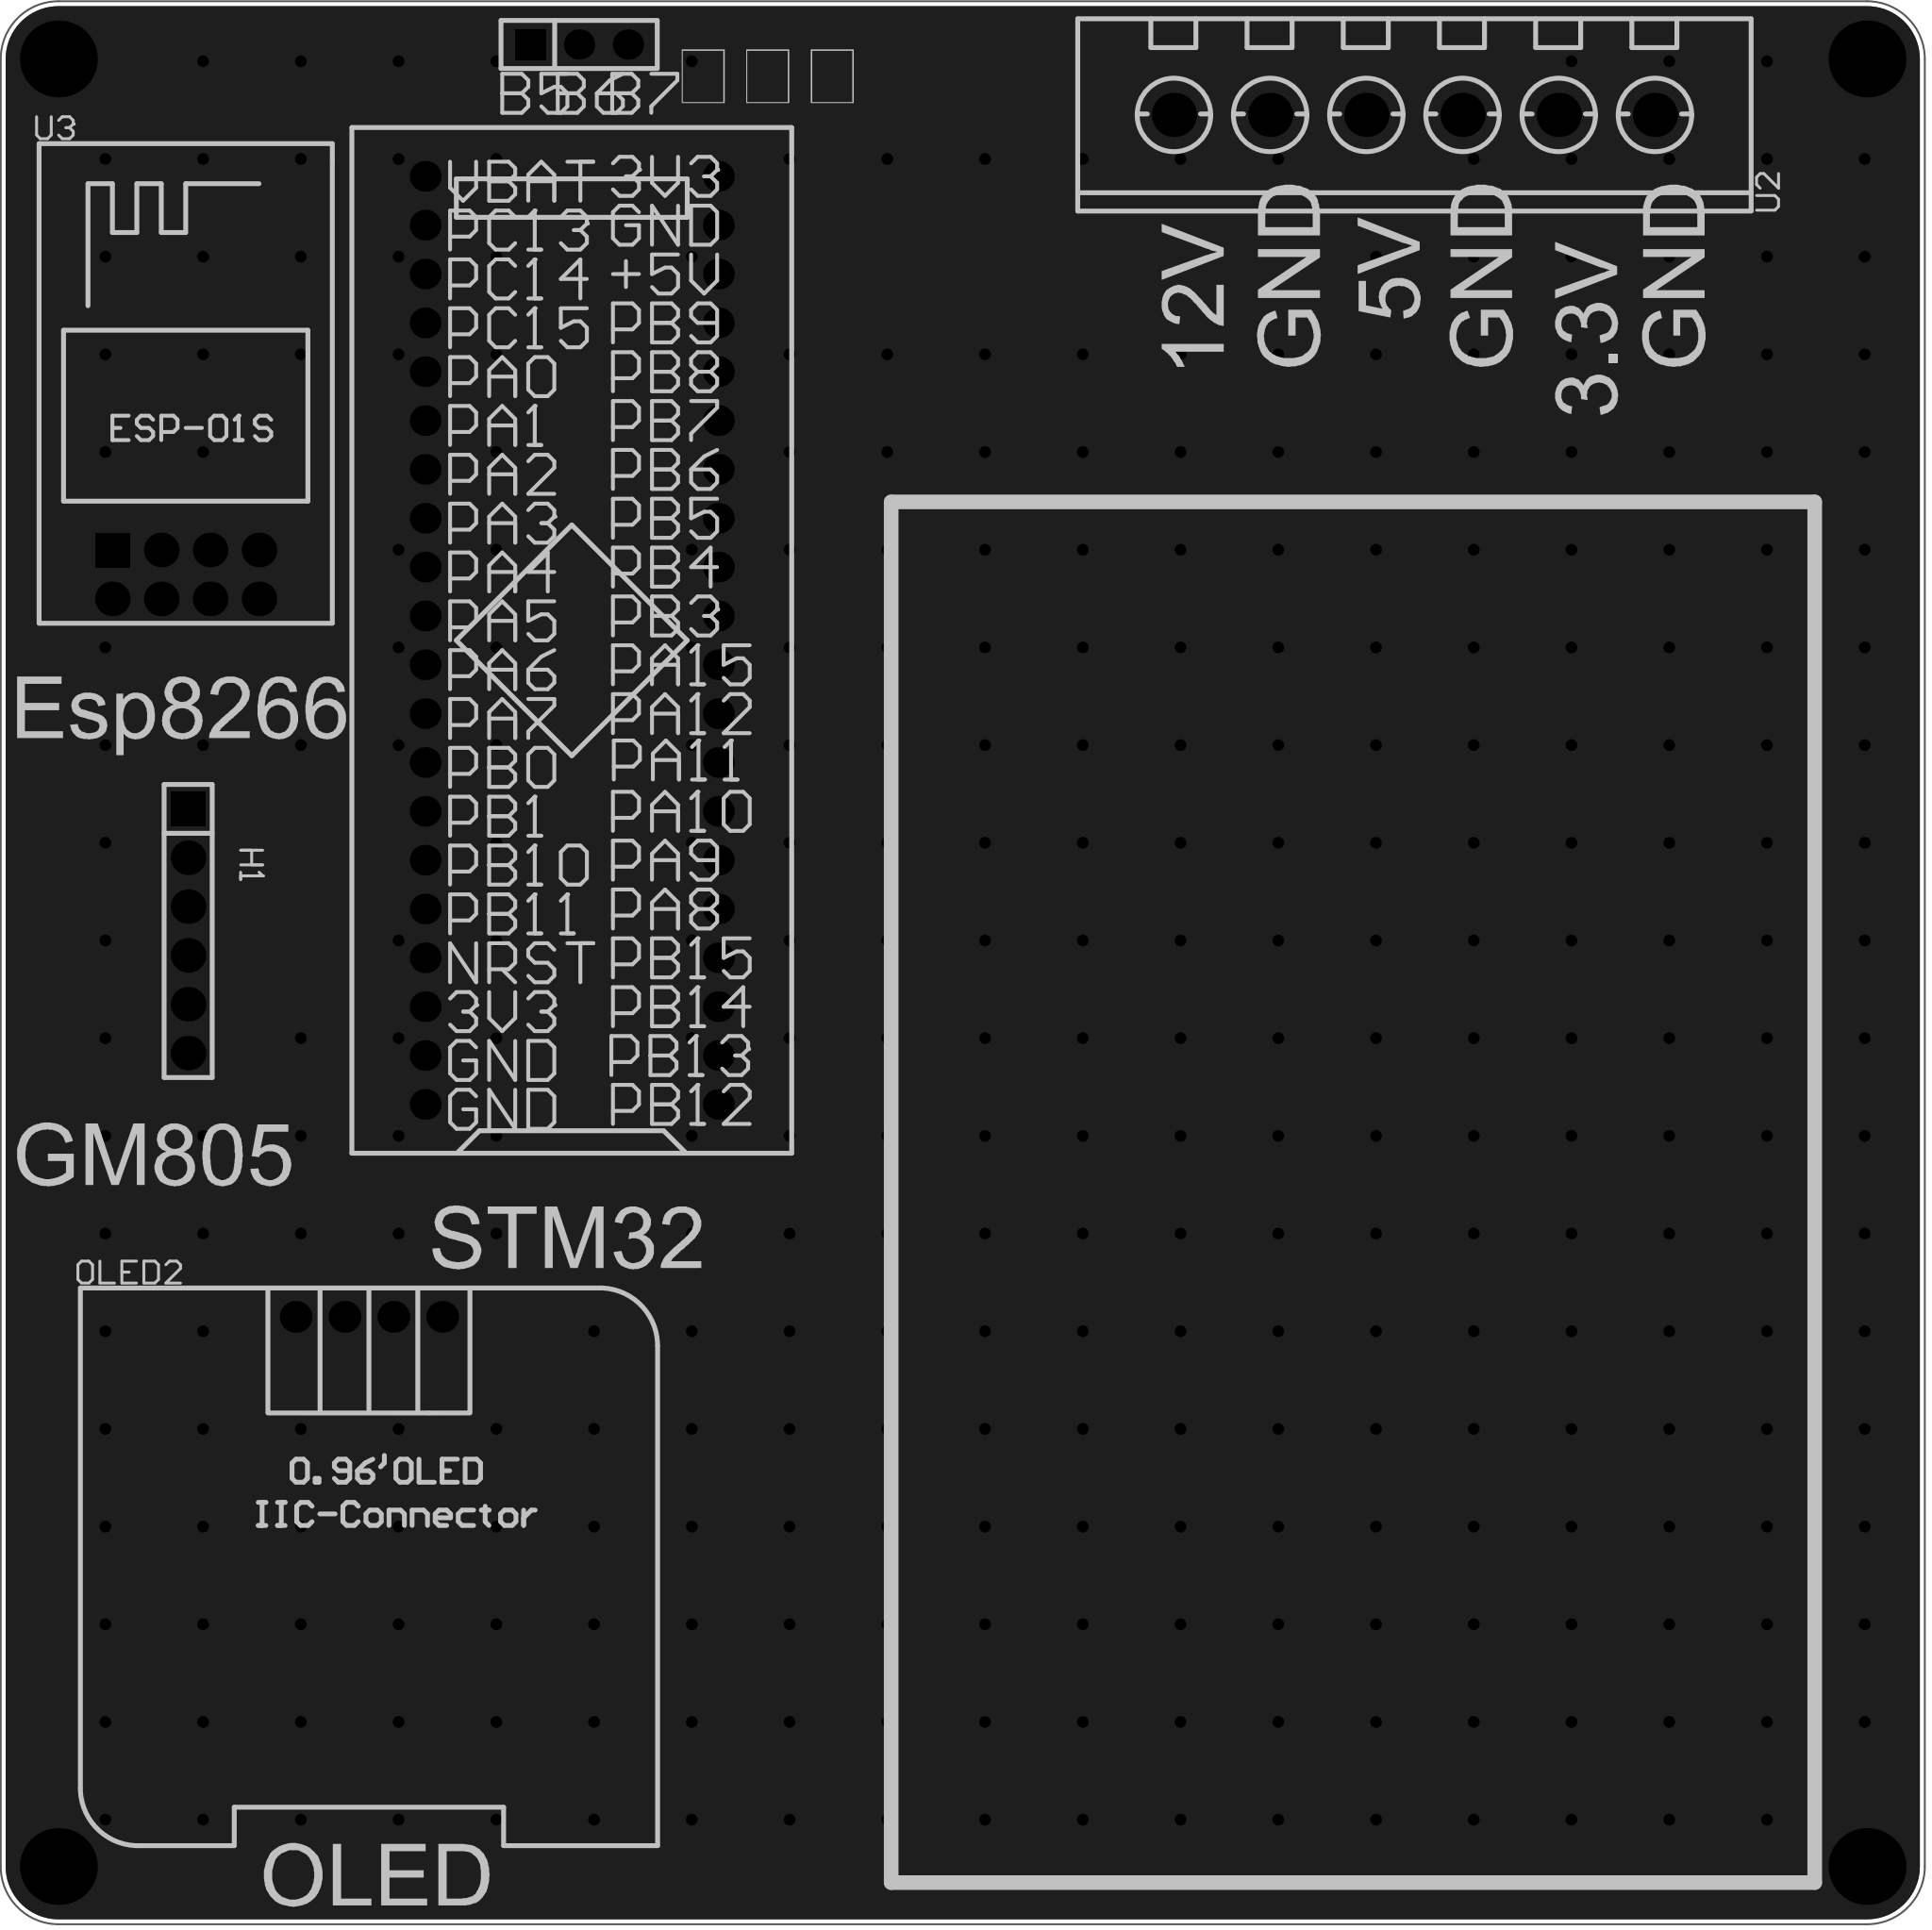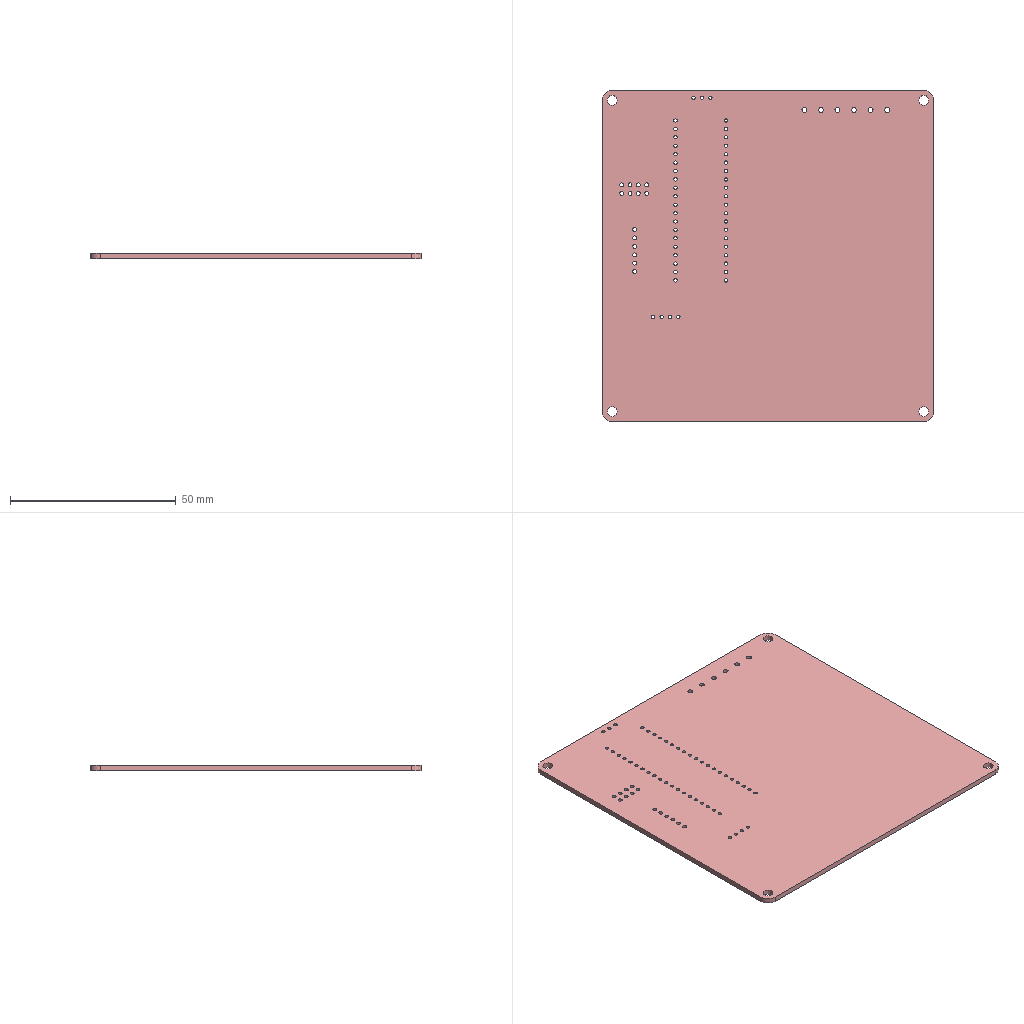Circuit board layout | Altium Designer | box 100 x 100 x 1.6 mm
Layer stack:
# Altium Designer layer stack of  (unit mm; dielectric type: 0 none, 1 core, 2 prepreg, 3 surface material)
index,name,kind,layer,copper_thickness_mm,dielectric_type,dielectric_thickness_mm,dielectric_material,dielectric_constant
0,Top Paste Mask Layer,other,,,,,,
1,Top Silkscreen Layer,other,,,,,,
2,Top Solder Mask Layer,dielectric,,,3,0.01,,3.3
3,Top Layer,copper,Top Layer,0.035,,,,
4,Dielectric1,dielectric,,,3,1.51,FR4,4.5
5,Bottom Layer,copper,Bottom Layer,0.035,,,,
6,Bottom Solder Mask Layer,dielectric,,,3,0.01,,3.3
7,Bottom Silkscreen Layer,other,,,,,,
8,Bottom Paste Mask Layer,other,,,,,,
# drill layer pairs: low layer,high layer
drill_pair,Top Layer,Bottom Layer
Part placement:
Designator,Comment,Layer,Footprint,Center-X(mm),Center-Y(mm),Rotation
U1,STM32F103C8T6-Card,TopLayer,CONN-TH_L53.3-W22.9_STM32F103C8T6-CARD,121.031,149.479,90
OLED2,,TopLayer,0.96OLED_4P,110.49,114.3,0
H9,,TopLayer,HDR-TH_3P-P2.54-V-F,121.412,180.467,0
U3,ESP-01S,TopLayer,WIFIM-TH_ESP-01S,100.965,152.908,0
U2,LG128V 5.08 6P180度螺丝用十字带一字型,TopLayer,CONN-TH_6P-P5.00_LG128V,164.826,176.804,180
H1,,TopLayer,HDR-TH_6P-P2.54-V-M-1,101.092,134.366,270
Pad and via stacks:
# Altium Designer via and pad stacks of  (unit mm). Each distinct definition once, with the count of objects using it.
# via: kind,start_layer,end_layer,hole_mm,diameter_mm,mode(0 simple;1 top-mid-bottom;2 full stack),diameter_per_layer,count,example_net
# pad: kind,layer,hole_mm,hole_type(0 round;1 square;2 slot),plating,top_size,top_shape(1 round;2 rect;3 octagon;9 rounded rect),mid_size,bottom_size,mode,footprint,size_per_layer,count,example
pad,Multi-Layer,3,0,plated,4x4,1,4x4,4x4,0,,,4,1
pad,Multi-Layer,1,0,plated,1.6x1.6,1,1.6x1.6,1.6x1.6,0,CONN-TH_L53.3-W22.9_STM32F103C8T6-CARD,,40,U1.1
pad,Multi-Layer,1,0,plated,1.65x1.65,1,1.65x1.65,1.65x1.65,0,0.96OLED_4P,,4,OLED2.4
pad,Multi-Layer,1.02,0,plated,1.575x1.575,1,1.575x1.575,1.575x1.575,0,HDR-TH_3P-P2.54-V-F,,2,H9.3
pad,Multi-Layer,1.02,0,plated,1.575x1.575,2,1.575x1.575,1.575x1.575,0,HDR-TH_3P-P2.54-V-F,,1,H9.1
pad,Multi-Layer,1.2,0,plated,1.8x1.8,2,1.8x1.8,1.8x1.8,0,WIFIM-TH_ESP-01S,,1,U3.1
pad,Multi-Layer,1.2,0,plated,1.8x1.8,1,1.8x1.8,1.8x1.8,0,WIFIM-TH_ESP-01S,,7,U3.2
pad,Multi-Layer,1.5,0,plated,2.3x2.3,1,2.3x2.3,2.3x2.3,0,CONN-TH_6P-P5.00_LG128V,,6,U2.1
pad,Multi-Layer,1.2,0,plated,1.8x1.8,1,1.8x1.8,1.8x1.8,0,HDR-TH_6P-P2.54-V-M-1,,5,H1.6
pad,Multi-Layer,1.2,0,plated,1.8x1.8,2,1.8x1.8,1.8x1.8,0,HDR-TH_6P-P2.54-V-M-1,,1,H1.1
via,Top Layer,Bottom Layer,0.3048,0.61,0,,311,GND
Copper pours:
name,layer,net,type(0 solid;1 hatched;2 none)
Bottom Layer-GND,Bottom Layer,GND,0
Top Layer-GND,Top Layer,GND,0
Design rules, without the lines most boards share:
# Altium Designer design rules of  (exported by Altium Designer, unit mm)
# columns: name | kind | enabled | priority | scope1 | scope2 | descriptor | typed fields (field=value)
Copper_copperRegion_copperThickness1oz | 0 | disabled | 4 | All | All | Clearance Constraint (Gap=5.984mil) (Disabled)(All),(All) | gap=0.152
Copper_copperRegion_copperThickness1oz_1 | 63 | disabled | 4 | All | All | Board Clearance Constraint (Gap=0mil) (Disabled)(All) |
Copper_copperRegion_Copper_copperRegion | 0 | disabled | 5 | All | All | Clearance Constraint (Gap=5.984mil) (Disabled)(All),(All) | gap=0.152
Copper_copperRegion_Copper_copperRegion_1 | 63 | disabled | 5 | All | All | Board Clearance Constraint (Gap=0mil) (Disabled)(All) |
copperThickness1oz | 0 | enabled | 6 | All | All | Clearance Constraint (Gap=5.984mil) (All),(All) | gap=0.152
copperThickness1oz_1 | 63 | enabled | 6 | All | All | Board Clearance Constraint (Gap=0mil) (All) |
copperRegion_copperThickness1oz | 20 | disabled | 1 | All | All | Polygon Connect Rule(Relief Connect )(Conductor Width=10mil) (Relief Angle=90 Angle) (Entries=4) (Air Gap Width=10mil) (Disabled)(All),(All) | connect_style(0=relief,1=direct,2=none)=0 relief_conductor_width=0.254 relief_entries=4
copperRegion_Copper_copperRegion | 20 | disabled | 2 | All | All | Polygon Connect Rule(Relief Connect )(Conductor Width=10mil) (Relief Angle=90 Angle) (Entries=4) (Air Gap Width=10mil) (Disabled)(All),(All) | connect_style(0=relief,1=direct,2=none)=0 relief_conductor_width=0.254 relief_entries=4
copperRegion | 20 | enabled | 3 | All | All | Polygon Connect Rule(Relief Connect )(Conductor Width=10mil) (Relief Angle=90 Angle) (Entries=4) (Air Gap Width=10mil) (All),(All) | connect_style(0=relief,1=direct,2=none)=0 relief_conductor_width=0.254 relief_entries=4